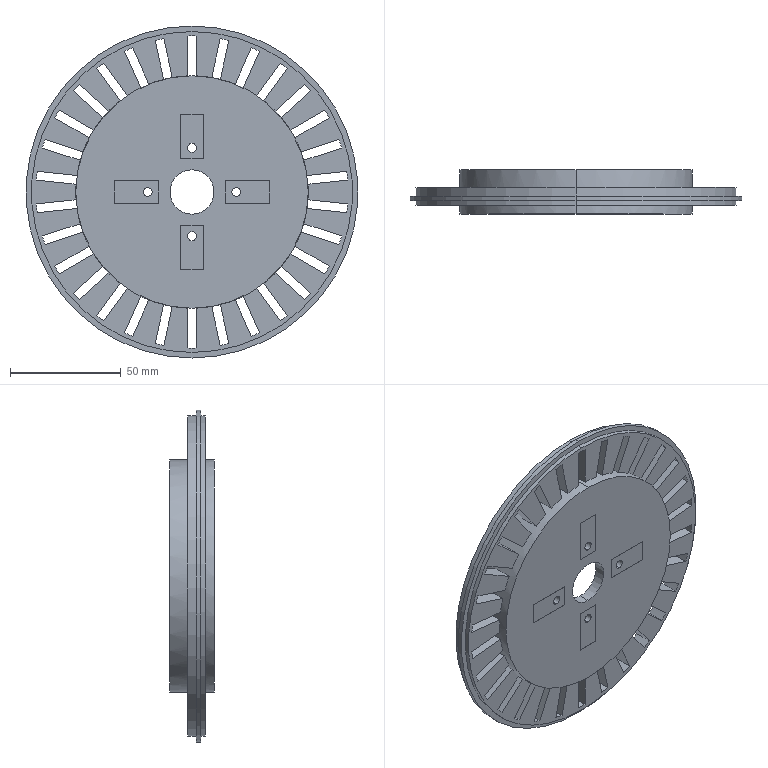Part | STEP file | Guide wheel mechanism revised.sldasm-Part-68 | 1 solid | 141 faces | box 150 x 20 x 150 mm | volume 149559 mm3 | plane 88 | cylinder 53 | commonest cylinder face diameters 141 x31 4 x8 145 x4 20 x2 70 x2 89 x2